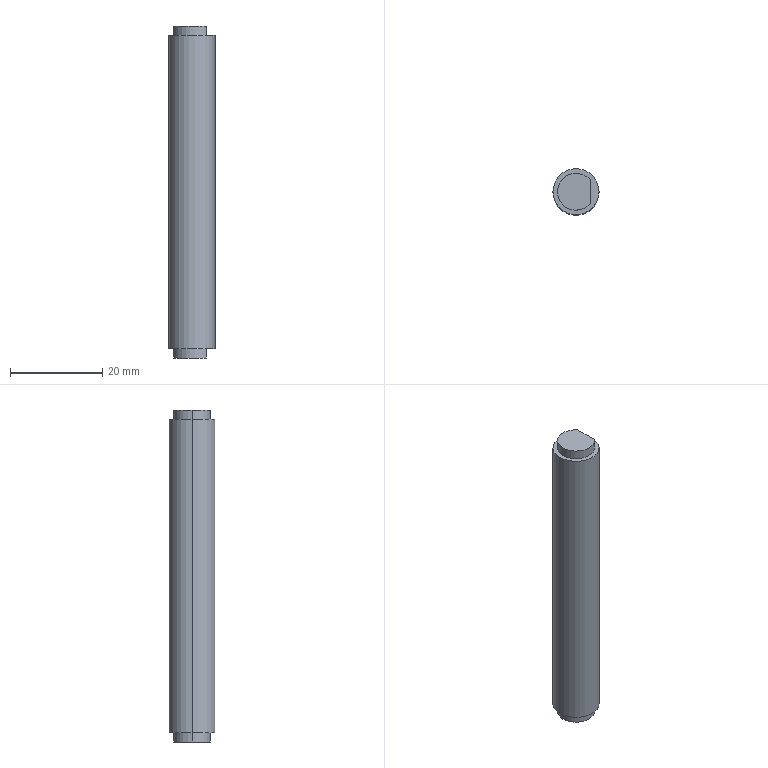Part | STEP file | 1 solid | 12 faces | box 10 x 10 x 72 mm | volume 5529 mm3 | cylinder 6 | plane 6 | commonest cylinder face diameters 8 x4 10 x2
STEP:
#1=CARTESIAN_POINT('',(0.,0.,0.));
#2=DIRECTION('',(0.,0.,1.));
#3=DIRECTION('',(1.,0.,0.));
#4=AXIS2_PLACEMENT_3D('',#1,#2,#3);
#5=CARTESIAN_POINT('',(34.355,10.689,0.));
#6=VERTEX_POINT('',#5);
#7=CARTESIAN_POINT('',(24.355,10.689,0.));
#8=VERTEX_POINT('',#7);
#9=CARTESIAN_POINT('',(29.355,10.689,0.));
#10=DIRECTION('',(0.,0.,1.));
#11=DIRECTION('',(1.,0.,0.));
#12=AXIS2_PLACEMENT_3D('',#9,#10,#11);
#13=CIRCLE('',#12,5.);
#14=CARTESIAN_POINT('',(29.355,10.689,34.));
#15=DIRECTION('',(0.,0.,1.));
#16=DIRECTION('',(1.,0.,0.));
#17=AXIS2_PLACEMENT_3D('',#14,#15,#16);
#18=CYLINDRICAL_SURFACE('',#17,5.);
#19=CARTESIAN_POINT('',(0.,-34.));
#20=DIRECTION('',(1.,0.));
#21=VECTOR('',#20,1.);
#22=LINE('',#19,#21);
#23=(GEOMETRIC_REPRESENTATION_CONTEXT(2)PARAMETRIC_REPRESENTATION_CONTEXT()REPRESENTATION_CONTEXT('',''));
#24=DEFINITIONAL_REPRESENTATION('',(#22),#23);
#25=PCURVE('',#18,#24);
#26=CARTESIAN_POINT('',(29.355,10.689,0.));
#27=DIRECTION('',(0.,0.,1.));
#28=DIRECTION('',(1.,0.,0.));
#29=AXIS2_PLACEMENT_3D('',#26,#27,#28);
#30=PLANE('',#29);
#31=CARTESIAN_POINT('',(0.,0.));
#32=DIRECTION('',(1.,0.));
#33=AXIS2_PLACEMENT_2D('',#31,#32);
#34=CIRCLE('',#33,5.);
#35=(GEOMETRIC_REPRESENTATION_CONTEXT(2)PARAMETRIC_REPRESENTATION_CONTEXT()REPRESENTATION_CONTEXT('',''));
#36=DEFINITIONAL_REPRESENTATION('',(#34),#35);
#37=PCURVE('',#30,#36);
#38=SURFACE_CURVE('',#13,(#25,#37),.PCURVE_S1.);
#39=EDGE_CURVE('',#6,#8,#38,.T.);
#40=ORIENTED_EDGE('',*,*,#39,.T.);
#41=CARTESIAN_POINT('',(24.355,10.689,68.));
#42=VERTEX_POINT('',#41);
#43=CARTESIAN_POINT('',(24.355,10.689,34.));
#44=DIRECTION('',(0.,0.,1.));
#45=VECTOR('',#44,1.);
#46=LINE('',#43,#45);
#47=CARTESIAN_POINT('',(3.142,0.));
#48=DIRECTION('',(0.,1.));
#49=VECTOR('',#48,1.);
#50=LINE('',#47,#49);
#51=(GEOMETRIC_REPRESENTATION_CONTEXT(2)PARAMETRIC_REPRESENTATION_CONTEXT()REPRESENTATION_CONTEXT('',''));
#52=DEFINITIONAL_REPRESENTATION('',(#50),#51);
#53=PCURVE('',#18,#52);
#54=CARTESIAN_POINT('',(29.355,10.689,34.));
#55=DIRECTION('',(0.,0.,1.));
#56=DIRECTION('',(1.,0.,0.));
#57=AXIS2_PLACEMENT_3D('',#54,#55,#56);
#58=CYLINDRICAL_SURFACE('',#57,5.);
#59=CARTESIAN_POINT('',(3.142,0.));
#60=DIRECTION('',(0.,1.));
#61=VECTOR('',#60,1.);
#62=LINE('',#59,#61);
#63=(GEOMETRIC_REPRESENTATION_CONTEXT(2)PARAMETRIC_REPRESENTATION_CONTEXT()REPRESENTATION_CONTEXT('',''));
#64=DEFINITIONAL_REPRESENTATION('',(#62),#63);
#65=PCURVE('',#58,#64);
#66=SURFACE_CURVE('',#46,(#53,#65),.PCURVE_S1.);
#67=EDGE_CURVE('',#8,#42,#66,.T.);
#68=ORIENTED_EDGE('',*,*,#67,.T.);
#69=CARTESIAN_POINT('',(34.355,10.689,68.));
#70=VERTEX_POINT('',#69);
#71=CARTESIAN_POINT('',(29.355,10.689,68.));
#72=DIRECTION('',(0.,0.,-1.));
#73=DIRECTION('',(1.,0.,0.));
#74=AXIS2_PLACEMENT_3D('',#71,#72,#73);
#75=CIRCLE('',#74,5.);
#76=CARTESIAN_POINT('',(6.283,34.));
#77=DIRECTION('',(-1.,0.));
#78=VECTOR('',#77,1.);
#79=LINE('',#76,#78);
#80=(GEOMETRIC_REPRESENTATION_CONTEXT(2)PARAMETRIC_REPRESENTATION_CONTEXT()REPRESENTATION_CONTEXT('',''));
#81=DEFINITIONAL_REPRESENTATION('',(#79),#80);
#82=PCURVE('',#18,#81);
#83=CARTESIAN_POINT('',(29.355,10.689,68.));
#84=DIRECTION('',(0.,0.,1.));
#85=DIRECTION('',(1.,0.,0.));
#86=AXIS2_PLACEMENT_3D('',#83,#84,#85);
#87=PLANE('',#86);
#88=CARTESIAN_POINT('',(5.,0.));
#89=CARTESIAN_POINT('',(5.,-8.66));
#90=CARTESIAN_POINT('',(-2.5,-4.33));
#91=CARTESIAN_POINT('',(-10.,0.));
#92=CARTESIAN_POINT('',(-2.5,4.33));
#93=CARTESIAN_POINT('',(5.,8.66));
#94=CARTESIAN_POINT('',(5.,0.));
#95=(BOUNDED_CURVE()B_SPLINE_CURVE(2,(#88,#89,#90,#91,#92,#93,#94),.UNSPECIFIED.,.T.,.F.)B_SPLINE_CURVE_WITH_KNOTS((1,2,2,2,2,1),(-2.094,0.,2.094,4.189,6.283,8.378),.UNSPECIFIED.)CURVE()GEOMETRIC_REPRESENTATION_ITEM()RATIONAL_B_SPLINE_CURVE((1.,0.5,1.,0.5,1.,0.5,1.))REPRESENTATION_ITEM(''));
#96=(GEOMETRIC_REPRESENTATION_CONTEXT(2)PARAMETRIC_REPRESENTATION_CONTEXT()REPRESENTATION_CONTEXT('',''));
#97=DEFINITIONAL_REPRESENTATION('',(#95),#96);
#98=PCURVE('',#87,#97);
#99=SURFACE_CURVE('',#75,(#82,#98),.PCURVE_S1.);
#100=EDGE_CURVE('',#42,#70,#99,.T.);
#101=ORIENTED_EDGE('',*,*,#100,.T.);
#102=CARTESIAN_POINT('',(34.355,10.689,34.));
#103=DIRECTION('',(0.,0.,1.));
#104=VECTOR('',#103,1.);
#105=LINE('',#102,#104);
#106=CARTESIAN_POINT('',(0.,0.));
#107=DIRECTION('',(0.,1.));
#108=VECTOR('',#107,1.);
#109=LINE('',#106,#108);
#110=(GEOMETRIC_REPRESENTATION_CONTEXT(2)PARAMETRIC_REPRESENTATION_CONTEXT()REPRESENTATION_CONTEXT('',''));
#111=DEFINITIONAL_REPRESENTATION('',(#109),#110);
#112=PCURVE('',#18,#111);
#113=CARTESIAN_POINT('',(6.283,0.));
#114=DIRECTION('',(0.,1.));
#115=VECTOR('',#114,1.);
#116=LINE('',#113,#115);
#117=(GEOMETRIC_REPRESENTATION_CONTEXT(2)PARAMETRIC_REPRESENTATION_CONTEXT()REPRESENTATION_CONTEXT('',''));
#118=DEFINITIONAL_REPRESENTATION('',(#116),#117);
#119=PCURVE('',#58,#118);
#120=SURFACE_CURVE('',#105,(#112,#119),.PCURVE_S1.);
#121=EDGE_CURVE('',#6,#70,#120,.T.);
#122=ORIENTED_EDGE('',*,*,#121,.F.);
#123=EDGE_LOOP('',(#40,#68,#101,#122));
#124=FACE_BOUND('',#123,.T.);
#125=ADVANCED_FACE('',(#124),#18,.T.);
#126=CARTESIAN_POINT('',(32.435,8.137,70.));
#127=VERTEX_POINT('',#126);
#128=CARTESIAN_POINT('',(25.355,10.689,70.));
#129=VERTEX_POINT('',#128);
#130=CARTESIAN_POINT('',(29.355,10.689,70.));
#131=DIRECTION('',(0.,0.,-1.));
#132=DIRECTION('',(-1.,0.,0.));
#133=AXIS2_PLACEMENT_3D('',#130,#131,#132);
#134=CIRCLE('',#133,4.);
#135=CARTESIAN_POINT('',(29.355,10.689,68.));
#136=DIRECTION('',(0.,0.,-1.));
#137=DIRECTION('',(-1.,0.,0.));
#138=AXIS2_PLACEMENT_3D('',#135,#136,#137);
#139=CYLINDRICAL_SURFACE('',#138,4.);
#140=CARTESIAN_POINT('',(0.,-2.));
#141=DIRECTION('',(1.,0.));
#142=VECTOR('',#141,1.);
#143=LINE('',#140,#142);
#144=(GEOMETRIC_REPRESENTATION_CONTEXT(2)PARAMETRIC_REPRESENTATION_CONTEXT()REPRESENTATION_CONTEXT('',''));
#145=DEFINITIONAL_REPRESENTATION('',(#143),#144);
#146=PCURVE('',#139,#145);
#147=CARTESIAN_POINT('',(29.375,10.689,70.));
#148=DIRECTION('',(0.,0.,1.));
#149=DIRECTION('',(1.,0.,0.));
#150=AXIS2_PLACEMENT_3D('',#147,#148,#149);
#151=PLANE('',#150);
#152=CARTESIAN_POINT('',(-4.021,0.));
#153=CARTESIAN_POINT('',(-4.021,6.928));
#154=CARTESIAN_POINT('',(1.979,3.464));
#155=CARTESIAN_POINT('',(7.979,0.));
#156=CARTESIAN_POINT('',(1.979,-3.464));
#157=CARTESIAN_POINT('',(-4.021,-6.928));
#158=CARTESIAN_POINT('',(-4.021,0.));
#159=(BOUNDED_CURVE()B_SPLINE_CURVE(2,(#152,#153,#154,#155,#156,#157,#158),.UNSPECIFIED.,.T.,.F.)B_SPLINE_CURVE_WITH_KNOTS((1,2,2,2,2,1),(-2.094,0.,2.094,4.189,6.283,8.378),.UNSPECIFIED.)CURVE()GEOMETRIC_REPRESENTATION_ITEM()RATIONAL_B_SPLINE_CURVE((1.,0.5,1.,0.5,1.,0.5,1.))REPRESENTATION_ITEM(''));
#160=(GEOMETRIC_REPRESENTATION_CONTEXT(2)PARAMETRIC_REPRESENTATION_CONTEXT()REPRESENTATION_CONTEXT('',''));
#161=DEFINITIONAL_REPRESENTATION('',(#159),#160);
#162=PCURVE('',#151,#161);
#163=SURFACE_CURVE('',#134,(#146,#162),.PCURVE_S1.);
#164=EDGE_CURVE('',#127,#129,#163,.T.);
#165=ORIENTED_EDGE('',*,*,#164,.T.);
#166=CARTESIAN_POINT('',(25.355,10.689,68.));
#167=VERTEX_POINT('',#166);
#168=CARTESIAN_POINT('',(25.355,10.689,68.));
#169=DIRECTION('',(0.,0.,-1.));
#170=VECTOR('',#169,1.);
#171=LINE('',#168,#170);
#172=CARTESIAN_POINT('',(6.283,0.));
#173=DIRECTION('',(0.,1.));
#174=VECTOR('',#173,1.);
#175=LINE('',#172,#174);
#176=(GEOMETRIC_REPRESENTATION_CONTEXT(2)PARAMETRIC_REPRESENTATION_CONTEXT()REPRESENTATION_CONTEXT('',''));
#177=DEFINITIONAL_REPRESENTATION('',(#175),#176);
#178=PCURVE('',#139,#177);
#179=CARTESIAN_POINT('',(29.355,10.689,68.));
#180=DIRECTION('',(0.,0.,-1.));
#181=DIRECTION('',(-1.,0.,0.));
#182=AXIS2_PLACEMENT_3D('',#179,#180,#181);
#183=CYLINDRICAL_SURFACE('',#182,4.);
#184=CARTESIAN_POINT('',(0.,0.));
#185=DIRECTION('',(0.,1.));
#186=VECTOR('',#185,1.);
#187=LINE('',#184,#186);
#188=(GEOMETRIC_REPRESENTATION_CONTEXT(2)PARAMETRIC_REPRESENTATION_CONTEXT()REPRESENTATION_CONTEXT('',''));
#189=DEFINITIONAL_REPRESENTATION('',(#187),#188);
#190=PCURVE('',#183,#189);
#191=SURFACE_CURVE('',#171,(#178,#190),.PCURVE_S1.);
#192=EDGE_CURVE('',#129,#167,#191,.T.);
#193=ORIENTED_EDGE('',*,*,#192,.T.);
#194=CARTESIAN_POINT('',(32.435,8.137,68.));
#195=VERTEX_POINT('',#194);
#196=CARTESIAN_POINT('',(29.355,10.689,68.));
#197=DIRECTION('',(0.,0.,-1.));
#198=DIRECTION('',(-1.,0.,0.));
#199=AXIS2_PLACEMENT_3D('',#196,#197,#198);
#200=CIRCLE('',#199,4.);
#201=CARTESIAN_POINT('',(0.,0.));
#202=DIRECTION('',(1.,0.));
#203=VECTOR('',#202,1.);
#204=LINE('',#201,#203);
#205=(GEOMETRIC_REPRESENTATION_CONTEXT(2)PARAMETRIC_REPRESENTATION_CONTEXT()REPRESENTATION_CONTEXT('',''));
#206=DEFINITIONAL_REPRESENTATION('',(#204),#205);
#207=PCURVE('',#139,#206);
#208=CARTESIAN_POINT('',(-4.,0.));
#209=CARTESIAN_POINT('',(-4.,6.928));
#210=CARTESIAN_POINT('',(2.,3.464));
#211=CARTESIAN_POINT('',(8.,0.));
#212=CARTESIAN_POINT('',(2.,-3.464));
#213=CARTESIAN_POINT('',(-4.,-6.928));
#214=CARTESIAN_POINT('',(-4.,0.));
#215=(BOUNDED_CURVE()B_SPLINE_CURVE(2,(#208,#209,#210,#211,#212,#213,#214),.UNSPECIFIED.,.T.,.F.)B_SPLINE_CURVE_WITH_KNOTS((1,2,2,2,2,1),(-2.094,0.,2.094,4.189,6.283,8.378),.UNSPECIFIED.)CURVE()GEOMETRIC_REPRESENTATION_ITEM()RATIONAL_B_SPLINE_CURVE((1.,0.5,1.,0.5,1.,0.5,1.))REPRESENTATION_ITEM(''));
#216=(GEOMETRIC_REPRESENTATION_CONTEXT(2)PARAMETRIC_REPRESENTATION_CONTEXT()REPRESENTATION_CONTEXT('',''));
#217=DEFINITIONAL_REPRESENTATION('',(#215),#216);
#218=PCURVE('',#87,#217);
#219=SURFACE_CURVE('',#200,(#207,#218),.PCURVE_S1.);
#220=EDGE_CURVE('',#195,#167,#219,.T.);
#221=ORIENTED_EDGE('',*,*,#220,.F.);
#222=CARTESIAN_POINT('',(32.435,8.137,68.));
#223=DIRECTION('',(0.,0.,1.));
#224=VECTOR('',#223,1.);
#225=LINE('',#222,#224);
#226=CARTESIAN_POINT('',(3.833,0.));
#227=DIRECTION('',(0.,-1.));
#228=VECTOR('',#227,1.);
#229=LINE('',#226,#228);
#230=(GEOMETRIC_REPRESENTATION_CONTEXT(2)PARAMETRIC_REPRESENTATION_CONTEXT()REPRESENTATION_CONTEXT('',''));
#231=DEFINITIONAL_REPRESENTATION('',(#229),#230);
#232=PCURVE('',#139,#231);
#233=CARTESIAN_POINT('',(32.435,13.24,68.));
#234=DIRECTION('',(-1.,0.,0.));
#235=DIRECTION('',(0.,-1.,0.));
#236=AXIS2_PLACEMENT_3D('',#233,#234,#235);
#237=PLANE('',#236);
#238=CARTESIAN_POINT('',(5.103,0.));
#239=DIRECTION('',(0.,1.));
#240=VECTOR('',#239,1.);
#241=LINE('',#238,#240);
#242=(GEOMETRIC_REPRESENTATION_CONTEXT(2)PARAMETRIC_REPRESENTATION_CONTEXT()REPRESENTATION_CONTEXT('',''));
#243=DEFINITIONAL_REPRESENTATION('',(#241),#242);
#244=PCURVE('',#237,#243);
#245=SURFACE_CURVE('',#225,(#232,#244),.PCURVE_S1.);
#246=EDGE_CURVE('',#195,#127,#245,.T.);
#247=ORIENTED_EDGE('',*,*,#246,.T.);
#248=EDGE_LOOP('',(#165,#193,#221,#247));
#249=FACE_BOUND('',#248,.T.);
#250=ADVANCED_FACE('',(#249),#139,.T.);
#251=CARTESIAN_POINT('',(32.435,8.137,0.));
#252=VERTEX_POINT('',#251);
#253=CARTESIAN_POINT('',(25.355,10.689,0.));
#254=VERTEX_POINT('',#253);
#255=CARTESIAN_POINT('',(29.355,10.689,0.));
#256=DIRECTION('',(0.,0.,-1.));
#257=DIRECTION('',(-1.,0.,0.));
#258=AXIS2_PLACEMENT_3D('',#255,#256,#257);
#259=CIRCLE('',#258,4.);
#260=CARTESIAN_POINT('',(29.355,10.689,0.));
#261=DIRECTION('',(0.,0.,-1.));
#262=DIRECTION('',(-1.,0.,0.));
#263=AXIS2_PLACEMENT_3D('',#260,#261,#262);
#264=CYLINDRICAL_SURFACE('',#263,4.);
#265=CARTESIAN_POINT('',(0.,0.));
#266=DIRECTION('',(1.,0.));
#267=VECTOR('',#266,1.);
#268=LINE('',#265,#267);
#269=(GEOMETRIC_REPRESENTATION_CONTEXT(2)PARAMETRIC_REPRESENTATION_CONTEXT()REPRESENTATION_CONTEXT('',''));
#270=DEFINITIONAL_REPRESENTATION('',(#268),#269);
#271=PCURVE('',#264,#270);
#272=CARTESIAN_POINT('',(-4.,0.));
#273=CARTESIAN_POINT('',(-4.,6.928));
#274=CARTESIAN_POINT('',(2.,3.464));
#275=CARTESIAN_POINT('',(8.,0.));
#276=CARTESIAN_POINT('',(2.,-3.464));
#277=CARTESIAN_POINT('',(-4.,-6.928));
#278=CARTESIAN_POINT('',(-4.,0.));
#279=(BOUNDED_CURVE()B_SPLINE_CURVE(2,(#272,#273,#274,#275,#276,#277,#278),.UNSPECIFIED.,.T.,.F.)B_SPLINE_CURVE_WITH_KNOTS((1,2,2,2,2,1),(-2.094,0.,2.094,4.189,6.283,8.378),.UNSPECIFIED.)CURVE()GEOMETRIC_REPRESENTATION_ITEM()RATIONAL_B_SPLINE_CURVE((1.,0.5,1.,0.5,1.,0.5,1.))REPRESENTATION_ITEM(''));
#280=(GEOMETRIC_REPRESENTATION_CONTEXT(2)PARAMETRIC_REPRESENTATION_CONTEXT()REPRESENTATION_CONTEXT('',''));
#281=DEFINITIONAL_REPRESENTATION('',(#279),#280);
#282=PCURVE('',#30,#281);
#283=SURFACE_CURVE('',#259,(#271,#282),.PCURVE_S1.);
#284=EDGE_CURVE('',#252,#254,#283,.T.);
#285=ORIENTED_EDGE('',*,*,#284,.T.);
#286=CARTESIAN_POINT('',(25.355,10.689,-2.));
#287=VERTEX_POINT('',#286);
#288=CARTESIAN_POINT('',(25.355,10.689,0.));
#289=DIRECTION('',(0.,0.,-1.));
#290=VECTOR('',#289,1.);
#291=LINE('',#288,#290);
#292=CARTESIAN_POINT('',(6.283,0.));
#293=DIRECTION('',(0.,1.));
#294=VECTOR('',#293,1.);
#295=LINE('',#292,#294);
#296=(GEOMETRIC_REPRESENTATION_CONTEXT(2)PARAMETRIC_REPRESENTATION_CONTEXT()REPRESENTATION_CONTEXT('',''));
#297=DEFINITIONAL_REPRESENTATION('',(#295),#296);
#298=PCURVE('',#264,#297);
#299=CARTESIAN_POINT('',(29.355,10.689,0.));
#300=DIRECTION('',(0.,0.,-1.));
#301=DIRECTION('',(-1.,0.,0.));
#302=AXIS2_PLACEMENT_3D('',#299,#300,#301);
#303=CYLINDRICAL_SURFACE('',#302,4.);
#304=CARTESIAN_POINT('',(0.,0.));
#305=DIRECTION('',(0.,1.));
#306=VECTOR('',#305,1.);
#307=LINE('',#304,#306);
#308=(GEOMETRIC_REPRESENTATION_CONTEXT(2)PARAMETRIC_REPRESENTATION_CONTEXT()REPRESENTATION_CONTEXT('',''));
#309=DEFINITIONAL_REPRESENTATION('',(#307),#308);
#310=PCURVE('',#303,#309);
#311=SURFACE_CURVE('',#291,(#298,#310),.PCURVE_S1.);
#312=EDGE_CURVE('',#254,#287,#311,.T.);
#313=ORIENTED_EDGE('',*,*,#312,.T.);
#314=CARTESIAN_POINT('',(32.435,8.137,-2.));
#315=VERTEX_POINT('',#314);
#316=CARTESIAN_POINT('',(29.355,10.689,-2.));
#317=DIRECTION('',(0.,0.,1.));
#318=DIRECTION('',(-1.,0.,0.));
#319=AXIS2_PLACEMENT_3D('',#316,#317,#318);
#320=CIRCLE('',#319,4.);
#321=CARTESIAN_POINT('',(6.283,2.));
#322=DIRECTION('',(-1.,0.));
#323=VECTOR('',#322,1.);
#324=LINE('',#321,#323);
#325=(GEOMETRIC_REPRESENTATION_CONTEXT(2)PARAMETRIC_REPRESENTATION_CONTEXT()REPRESENTATION_CONTEXT('',''));
#326=DEFINITIONAL_REPRESENTATION('',(#324),#325);
#327=PCURVE('',#264,#326);
#328=CARTESIAN_POINT('',(29.375,10.689,-2.));
#329=DIRECTION('',(0.,0.,1.));
#330=DIRECTION('',(1.,0.,0.));
#331=AXIS2_PLACEMENT_3D('',#328,#329,#330);
#332=PLANE('',#331);
#333=CARTESIAN_POINT('',(-0.02072,0.));
#334=DIRECTION('',(-1.,0.));
#335=AXIS2_PLACEMENT_2D('',#333,#334);
#336=CIRCLE('',#335,4.);
#337=(GEOMETRIC_REPRESENTATION_CONTEXT(2)PARAMETRIC_REPRESENTATION_CONTEXT()REPRESENTATION_CONTEXT('',''));
#338=DEFINITIONAL_REPRESENTATION('',(#336),#337);
#339=PCURVE('',#332,#338);
#340=SURFACE_CURVE('',#320,(#327,#339),.PCURVE_S1.);
#341=EDGE_CURVE('',#287,#315,#340,.T.);
#342=ORIENTED_EDGE('',*,*,#341,.T.);
#343=CARTESIAN_POINT('',(32.435,8.137,0.));
#344=DIRECTION('',(0.,0.,-1.));
#345=VECTOR('',#344,1.);
#346=LINE('',#343,#345);
#347=CARTESIAN_POINT('',(3.833,0.));
#348=DIRECTION('',(0.,1.));
#349=VECTOR('',#348,1.);
#350=LINE('',#347,#349);
#351=(GEOMETRIC_REPRESENTATION_CONTEXT(2)PARAMETRIC_REPRESENTATION_CONTEXT()REPRESENTATION_CONTEXT('',''));
#352=DEFINITIONAL_REPRESENTATION('',(#350),#351);
#353=PCURVE('',#264,#352);
#354=CARTESIAN_POINT('',(32.435,13.24,0.));
#355=DIRECTION('',(1.,0.,0.));
#356=DIRECTION('',(0.,1.,0.));
#357=AXIS2_PLACEMENT_3D('',#354,#355,#356);
#358=PLANE('',#357);
#359=CARTESIAN_POINT('',(-5.103,0.));
#360=DIRECTION('',(0.,-1.));
#361=VECTOR('',#360,1.);
#362=LINE('',#359,#361);
#363=(GEOMETRIC_REPRESENTATION_CONTEXT(2)PARAMETRIC_REPRESENTATION_CONTEXT()REPRESENTATION_CONTEXT('',''));
#364=DEFINITIONAL_REPRESENTATION('',(#362),#363);
#365=PCURVE('',#358,#364);
#366=SURFACE_CURVE('',#346,(#353,#365),.PCURVE_S1.);
#367=EDGE_CURVE('',#252,#315,#366,.T.);
#368=ORIENTED_EDGE('',*,*,#367,.F.);
#369=EDGE_LOOP('',(#285,#313,#342,#368));
#370=FACE_BOUND('',#369,.T.);
#371=ADVANCED_FACE('',(#370),#264,.T.);
#372=ORIENTED_EDGE('',*,*,#67,.F.);
#373=CARTESIAN_POINT('',(29.355,10.689,0.));
#374=DIRECTION('',(0.,0.,1.));
#375=DIRECTION('',(1.,0.,0.));
#376=AXIS2_PLACEMENT_3D('',#373,#374,#375);
#377=CIRCLE('',#376,5.);
#378=CARTESIAN_POINT('',(0.,-34.));
#379=DIRECTION('',(1.,0.));
#380=VECTOR('',#379,1.);
#381=LINE('',#378,#380);
#382=(GEOMETRIC_REPRESENTATION_CONTEXT(2)PARAMETRIC_REPRESENTATION_CONTEXT()REPRESENTATION_CONTEXT('',''));
#383=DEFINITIONAL_REPRESENTATION('',(#381),#382);
#384=PCURVE('',#58,#383);
#385=CARTESIAN_POINT('',(0.,0.));
#386=DIRECTION('',(1.,0.));
#387=AXIS2_PLACEMENT_2D('',#385,#386);
#388=CIRCLE('',#387,5.);
#389=(GEOMETRIC_REPRESENTATION_CONTEXT(2)PARAMETRIC_REPRESENTATION_CONTEXT()REPRESENTATION_CONTEXT('',''));
#390=DEFINITIONAL_REPRESENTATION('',(#388),#389);
#391=PCURVE('',#30,#390);
#392=SURFACE_CURVE('',#377,(#384,#391),.PCURVE_S1.);
#393=EDGE_CURVE('',#8,#6,#392,.T.);
#394=ORIENTED_EDGE('',*,*,#393,.T.);
#395=ORIENTED_EDGE('',*,*,#121,.T.);
#396=CARTESIAN_POINT('',(29.355,10.689,68.));
#397=DIRECTION('',(0.,0.,-1.));
#398=DIRECTION('',(1.,0.,0.));
#399=AXIS2_PLACEMENT_3D('',#396,#397,#398);
#400=CIRCLE('',#399,5.);
#401=CARTESIAN_POINT('',(6.283,34.));
#402=DIRECTION('',(-1.,0.));
#403=VECTOR('',#402,1.);
#404=LINE('',#401,#403);
#405=(GEOMETRIC_REPRESENTATION_CONTEXT(2)PARAMETRIC_REPRESENTATION_CONTEXT()REPRESENTATION_CONTEXT('',''));
#406=DEFINITIONAL_REPRESENTATION('',(#404),#405);
#407=PCURVE('',#58,#406);
#408=CARTESIAN_POINT('',(5.,0.));
#409=CARTESIAN_POINT('',(5.,-8.66));
#410=CARTESIAN_POINT('',(-2.5,-4.33));
#411=CARTESIAN_POINT('',(-10.,0.));
#412=CARTESIAN_POINT('',(-2.5,4.33));
#413=CARTESIAN_POINT('',(5.,8.66));
#414=CARTESIAN_POINT('',(5.,0.));
#415=(BOUNDED_CURVE()B_SPLINE_CURVE(2,(#408,#409,#410,#411,#412,#413,#414),.UNSPECIFIED.,.T.,.F.)B_SPLINE_CURVE_WITH_KNOTS((1,2,2,2,2,1),(-2.094,0.,2.094,4.189,6.283,8.378),.UNSPECIFIED.)CURVE()GEOMETRIC_REPRESENTATION_ITEM()RATIONAL_B_SPLINE_CURVE((1.,0.5,1.,0.5,1.,0.5,1.))REPRESENTATION_ITEM(''));
#416=(GEOMETRIC_REPRESENTATION_CONTEXT(2)PARAMETRIC_REPRESENTATION_CONTEXT()REPRESENTATION_CONTEXT('',''));
#417=DEFINITIONAL_REPRESENTATION('',(#415),#416);
#418=PCURVE('',#87,#417);
#419=SURFACE_CURVE('',#400,(#407,#418),.PCURVE_S1.);
#420=EDGE_CURVE('',#70,#42,#419,.T.);
#421=ORIENTED_EDGE('',*,*,#420,.T.);
#422=EDGE_LOOP('',(#372,#394,#395,#421));
#423=FACE_BOUND('',#422,.T.);
#424=ADVANCED_FACE('',(#423),#58,.T.);
#425=ORIENTED_EDGE('',*,*,#420,.F.);
#426=ORIENTED_EDGE('',*,*,#100,.F.);
#427=EDGE_LOOP('',(#425,#426));
#428=FACE_BOUND('',#427,.T.);
#429=CARTESIAN_POINT('',(32.435,13.24,68.));
#430=VERTEX_POINT('',#429);
#431=CARTESIAN_POINT('',(32.435,10.689,68.));
#432=DIRECTION('',(0.,-1.,0.));
#433=VECTOR('',#432,1.);
#434=LINE('',#431,#433);
#435=CARTESIAN_POINT('',(3.08,0.));
#436=DIRECTION('',(0.,-1.));
#437=VECTOR('',#436,1.);
#438=LINE('',#435,#437);
#439=(GEOMETRIC_REPRESENTATION_CONTEXT(2)PARAMETRIC_REPRESENTATION_CONTEXT()REPRESENTATION_CONTEXT('',''));
#440=DEFINITIONAL_REPRESENTATION('',(#438),#439);
#441=PCURVE('',#87,#440);
#442=CARTESIAN_POINT('',(2.552,0.));
#443=DIRECTION('',(1.,0.));
#444=VECTOR('',#443,1.);
#445=LINE('',#442,#444);
#446=(GEOMETRIC_REPRESENTATION_CONTEXT(2)PARAMETRIC_REPRESENTATION_CONTEXT()REPRESENTATION_CONTEXT('',''));
#447=DEFINITIONAL_REPRESENTATION('',(#445),#446);
#448=PCURVE('',#237,#447);
#449=SURFACE_CURVE('',#434,(#441,#448),.PCURVE_S1.);
#450=EDGE_CURVE('',#430,#195,#449,.T.);
#451=ORIENTED_EDGE('',*,*,#450,.T.);
#452=ORIENTED_EDGE('',*,*,#220,.T.);
#453=CARTESIAN_POINT('',(29.355,10.689,68.));
#454=DIRECTION('',(0.,0.,-1.));
#455=DIRECTION('',(-1.,0.,0.));
#456=AXIS2_PLACEMENT_3D('',#453,#454,#455);
#457=CIRCLE('',#456,4.);
#458=CARTESIAN_POINT('',(-4.,0.));
#459=CARTESIAN_POINT('',(-4.,6.928));
#460=CARTESIAN_POINT('',(2.,3.464));
#461=CARTESIAN_POINT('',(8.,0.));
#462=CARTESIAN_POINT('',(2.,-3.464));
#463=CARTESIAN_POINT('',(-4.,-6.928));
#464=CARTESIAN_POINT('',(-4.,0.));
#465=(BOUNDED_CURVE()B_SPLINE_CURVE(2,(#458,#459,#460,#461,#462,#463,#464),.UNSPECIFIED.,.T.,.F.)B_SPLINE_CURVE_WITH_KNOTS((1,2,2,2,2,1),(-2.094,0.,2.094,4.189,6.283,8.378),.UNSPECIFIED.)CURVE()GEOMETRIC_REPRESENTATION_ITEM()RATIONAL_B_SPLINE_CURVE((1.,0.5,1.,0.5,1.,0.5,1.))REPRESENTATION_ITEM(''));
#466=(GEOMETRIC_REPRESENTATION_CONTEXT(2)PARAMETRIC_REPRESENTATION_CONTEXT()REPRESENTATION_CONTEXT('',''));
#467=DEFINITIONAL_REPRESENTATION('',(#465),#466);
#468=PCURVE('',#87,#467);
#469=CARTESIAN_POINT('',(0.,0.));
#470=DIRECTION('',(1.,0.));
#471=VECTOR('',#470,1.);
#472=LINE('',#469,#471);
#473=(GEOMETRIC_REPRESENTATION_CONTEXT(2)PARAMETRIC_REPRESENTATION_CONTEXT()REPRESENTATION_CONTEXT('',''));
#474=DEFINITIONAL_REPRESENTATION('',(#472),#473);
#475=PCURVE('',#183,#474);
#476=SURFACE_CURVE('',#457,(#468,#475),.PCURVE_S1.);
#477=EDGE_CURVE('',#167,#430,#476,.T.);
#478=ORIENTED_EDGE('',*,*,#477,.T.);
#479=EDGE_LOOP('',(#451,#452,#478));
#480=FACE_BOUND('',#479,.T.);
#481=ADVANCED_FACE('',(#428,#480),#87,.T.);
#482=ORIENTED_EDGE('',*,*,#39,.F.);
#483=ORIENTED_EDGE('',*,*,#393,.F.);
#484=EDGE_LOOP('',(#482,#483));
#485=FACE_BOUND('',#484,.T.);
#486=ORIENTED_EDGE('',*,*,#284,.F.);
#487=CARTESIAN_POINT('',(32.435,13.24,0.));
#488=VERTEX_POINT('',#487);
#489=CARTESIAN_POINT('',(32.435,10.689,0.));
#490=DIRECTION('',(0.,-1.,0.));
#491=VECTOR('',#490,1.);
#492=LINE('',#489,#491);
#493=CARTESIAN_POINT('',(3.08,0.));
#494=DIRECTION('',(0.,-1.));
#495=VECTOR('',#494,1.);
#496=LINE('',#493,#495);
#497=(GEOMETRIC_REPRESENTATION_CONTEXT(2)PARAMETRIC_REPRESENTATION_CONTEXT()REPRESENTATION_CONTEXT('',''));
#498=DEFINITIONAL_REPRESENTATION('',(#496),#497);
#499=PCURVE('',#30,#498);
#500=CARTESIAN_POINT('',(-2.552,0.));
#501=DIRECTION('',(-1.,0.));
#502=VECTOR('',#501,1.);
#503=LINE('',#500,#502);
#504=(GEOMETRIC_REPRESENTATION_CONTEXT(2)PARAMETRIC_REPRESENTATION_CONTEXT()REPRESENTATION_CONTEXT('',''));
#505=DEFINITIONAL_REPRESENTATION('',(#503),#504);
#506=PCURVE('',#358,#505);
#507=SURFACE_CURVE('',#492,(#499,#506),.PCURVE_S1.);
#508=EDGE_CURVE('',#488,#252,#507,.T.);
#509=ORIENTED_EDGE('',*,*,#508,.F.);
#510=CARTESIAN_POINT('',(29.355,10.689,0.));
#511=DIRECTION('',(0.,0.,-1.));
#512=DIRECTION('',(-1.,0.,0.));
#513=AXIS2_PLACEMENT_3D('',#510,#511,#512);
#514=CIRCLE('',#513,4.);
#515=CARTESIAN_POINT('',(-4.,0.));
#516=CARTESIAN_POINT('',(-4.,6.928));
#517=CARTESIAN_POINT('',(2.,3.464));
#518=CARTESIAN_POINT('',(8.,0.));
#519=CARTESIAN_POINT('',(2.,-3.464));
#520=CARTESIAN_POINT('',(-4.,-6.928));
#521=CARTESIAN_POINT('',(-4.,0.));
#522=(BOUNDED_CURVE()B_SPLINE_CURVE(2,(#515,#516,#517,#518,#519,#520,#521),.UNSPECIFIED.,.T.,.F.)B_SPLINE_CURVE_WITH_KNOTS((1,2,2,2,2,1),(-2.094,0.,2.094,4.189,6.283,8.378),.UNSPECIFIED.)CURVE()GEOMETRIC_REPRESENTATION_ITEM()RATIONAL_B_SPLINE_CURVE((1.,0.5,1.,0.5,1.,0.5,1.))REPRESENTATION_ITEM(''));
#523=(GEOMETRIC_REPRESENTATION_CONTEXT(2)PARAMETRIC_REPRESENTATION_CONTEXT()REPRESENTATION_CONTEXT('',''));
#524=DEFINITIONAL_REPRESENTATION('',(#522),#523);
#525=PCURVE('',#30,#524);
#526=CARTESIAN_POINT('',(0.,0.));
#527=DIRECTION('',(1.,0.));
#528=VECTOR('',#527,1.);
#529=LINE('',#526,#528);
#530=(GEOMETRIC_REPRESENTATION_CONTEXT(2)PARAMETRIC_REPRESENTATION_CONTEXT()REPRESENTATION_CONTEXT('',''));
#531=DEFINITIONAL_REPRESENTATION('',(#529),#530);
#532=PCURVE('',#303,#531);
#533=SURFACE_CURVE('',#514,(#525,#532),.PCURVE_S1.);
#534=EDGE_CURVE('',#254,#488,#533,.T.);
#535=ORIENTED_EDGE('',*,*,#534,.F.);
#536=EDGE_LOOP('',(#486,#509,#535));
#537=FACE_BOUND('',#536,.T.);
#538=ADVANCED_FACE('',(#485,#537),#30,.F.);
#539=ORIENTED_EDGE('',*,*,#192,.F.);
#540=CARTESIAN_POINT('',(32.435,13.24,70.));
#541=VERTEX_POINT('',#540);
#542=CARTESIAN_POINT('',(29.355,10.689,70.));
#543=DIRECTION('',(0.,0.,-1.));
#544=DIRECTION('',(-1.,0.,0.));
#545=AXIS2_PLACEMENT_3D('',#542,#543,#544);
#546=CIRCLE('',#545,4.);
#547=CARTESIAN_POINT('',(0.,-2.));
#548=DIRECTION('',(1.,0.));
#549=VECTOR('',#548,1.);
#550=LINE('',#547,#549);
#551=(GEOMETRIC_REPRESENTATION_CONTEXT(2)PARAMETRIC_REPRESENTATION_CONTEXT()REPRESENTATION_CONTEXT('',''));
#552=DEFINITIONAL_REPRESENTATION('',(#550),#551);
#553=PCURVE('',#183,#552);
#554=CARTESIAN_POINT('',(-4.021,0.));
#555=CARTESIAN_POINT('',(-4.021,6.928));
#556=CARTESIAN_POINT('',(1.979,3.464));
#557=CARTESIAN_POINT('',(7.979,0.));
#558=CARTESIAN_POINT('',(1.979,-3.464));
#559=CARTESIAN_POINT('',(-4.021,-6.928));
#560=CARTESIAN_POINT('',(-4.021,0.));
#561=(BOUNDED_CURVE()B_SPLINE_CURVE(2,(#554,#555,#556,#557,#558,#559,#560),.UNSPECIFIED.,.T.,.F.)B_SPLINE_CURVE_WITH_KNOTS((1,2,2,2,2,1),(-2.094,0.,2.094,4.189,6.283,8.378),.UNSPECIFIED.)CURVE()GEOMETRIC_REPRESENTATION_ITEM()RATIONAL_B_SPLINE_CURVE((1.,0.5,1.,0.5,1.,0.5,1.))REPRESENTATION_ITEM(''));
#562=(GEOMETRIC_REPRESENTATION_CONTEXT(2)PARAMETRIC_REPRESENTATION_CONTEXT()REPRESENTATION_CONTEXT('',''));
#563=DEFINITIONAL_REPRESENTATION('',(#561),#562);
#564=PCURVE('',#151,#563);
#565=SURFACE_CURVE('',#546,(#553,#564),.PCURVE_S1.);
#566=EDGE_CURVE('',#129,#541,#565,.T.);
#567=ORIENTED_EDGE('',*,*,#566,.T.);
#568=CARTESIAN_POINT('',(32.435,13.24,68.));
#569=DIRECTION('',(0.,0.,-1.));
#570=VECTOR('',#569,1.);
#571=LINE('',#568,#570);
#572=CARTESIAN_POINT('',(2.45,0.));
#573=DIRECTION('',(0.,1.));
#574=VECTOR('',#573,1.);
#575=LINE('',#572,#574);
#576=(GEOMETRIC_REPRESENTATION_CONTEXT(2)PARAMETRIC_REPRESENTATION_CONTEXT()REPRESENTATION_CONTEXT('',''));
#577=DEFINITIONAL_REPRESENTATION('',(#575),#576);
#578=PCURVE('',#183,#577);
#579=CARTESIAN_POINT('',(0.,0.));
#580=DIRECTION('',(0.,-1.));
#581=VECTOR('',#580,1.);
#582=LINE('',#579,#581);
#583=(GEOMETRIC_REPRESENTATION_CONTEXT(2)PARAMETRIC_REPRESENTATION_CONTEXT()REPRESENTATION_CONTEXT('',''));
#584=DEFINITIONAL_REPRESENTATION('',(#582),#583);
#585=PCURVE('',#237,#584);
#586=SURFACE_CURVE('',#571,(#578,#585),.PCURVE_S1.);
#587=EDGE_CURVE('',#541,#430,#586,.T.);
#588=ORIENTED_EDGE('',*,*,#587,.T.);
#589=ORIENTED_EDGE('',*,*,#477,.F.);
#590=EDGE_LOOP('',(#539,#567,#588,#589));
#591=FACE_BOUND('',#590,.T.);
#592=ADVANCED_FACE('',(#591),#183,.T.);
#593=ORIENTED_EDGE('',*,*,#587,.F.);
#594=CARTESIAN_POINT('',(32.435,13.24,70.));
#595=DIRECTION('',(0.,1.,0.));
#596=VECTOR('',#595,1.);
#597=LINE('',#594,#596);
#598=CARTESIAN_POINT('',(0.,2.));
#599=DIRECTION('',(-1.,0.));
#600=VECTOR('',#599,1.);
#601=LINE('',#598,#600);
#602=(GEOMETRIC_REPRESENTATION_CONTEXT(2)PARAMETRIC_REPRESENTATION_CONTEXT()REPRESENTATION_CONTEXT('',''));
#603=DEFINITIONAL_REPRESENTATION('',(#601),#602);
#604=PCURVE('',#237,#603);
#605=CARTESIAN_POINT('',(3.06,2.552));
#606=DIRECTION('',(0.,1.));
#607=VECTOR('',#606,1.);
#608=LINE('',#605,#607);
#609=(GEOMETRIC_REPRESENTATION_CONTEXT(2)PARAMETRIC_REPRESENTATION_CONTEXT()REPRESENTATION_CONTEXT('',''));
#610=DEFINITIONAL_REPRESENTATION('',(#608),#609);
#611=PCURVE('',#151,#610);
#612=SURFACE_CURVE('',#597,(#604,#611),.PCURVE_S1.);
#613=EDGE_CURVE('',#127,#541,#612,.T.);
#614=ORIENTED_EDGE('',*,*,#613,.F.);
#615=ORIENTED_EDGE('',*,*,#246,.F.);
#616=ORIENTED_EDGE('',*,*,#450,.F.);
#617=EDGE_LOOP('',(#593,#614,#615,#616));
#618=FACE_BOUND('',#617,.T.);
#619=ADVANCED_FACE('',(#618),#237,.F.);
#620=CARTESIAN_POINT('',(32.435,13.24,-2.));
#621=VERTEX_POINT('',#620);
#622=CARTESIAN_POINT('',(32.435,13.24,-2.));
#623=DIRECTION('',(0.,1.,0.));
#624=VECTOR('',#623,1.);
#625=LINE('',#622,#624);
#626=CARTESIAN_POINT('',(0.,-2.));
#627=DIRECTION('',(1.,0.));
#628=VECTOR('',#627,1.);
#629=LINE('',#626,#628);
#630=(GEOMETRIC_REPRESENTATION_CONTEXT(2)PARAMETRIC_REPRESENTATION_CONTEXT()REPRESENTATION_CONTEXT('',''));
#631=DEFINITIONAL_REPRESENTATION('',(#629),#630);
#632=PCURVE('',#358,#631);
#633=CARTESIAN_POINT('',(3.06,2.552));
#634=DIRECTION('',(0.,1.));
#635=VECTOR('',#634,1.);
#636=LINE('',#633,#635);
#637=(GEOMETRIC_REPRESENTATION_CONTEXT(2)PARAMETRIC_REPRESENTATION_CONTEXT()REPRESENTATION_CONTEXT('',''));
#638=DEFINITIONAL_REPRESENTATION('',(#636),#637);
#639=PCURVE('',#332,#638);
#640=SURFACE_CURVE('',#625,(#632,#639),.PCURVE_S1.);
#641=EDGE_CURVE('',#315,#621,#640,.T.);
#642=ORIENTED_EDGE('',*,*,#641,.T.);
#643=CARTESIAN_POINT('',(32.435,13.24,0.));
#644=DIRECTION('',(0.,0.,1.));
#645=VECTOR('',#644,1.);
#646=LINE('',#643,#645);
#647=CARTESIAN_POINT('',(0.,0.));
#648=DIRECTION('',(0.,1.));
#649=VECTOR('',#648,1.);
#650=LINE('',#647,#649);
#651=(GEOMETRIC_REPRESENTATION_CONTEXT(2)PARAMETRIC_REPRESENTATION_CONTEXT()REPRESENTATION_CONTEXT('',''));
#652=DEFINITIONAL_REPRESENTATION('',(#650),#651);
#653=PCURVE('',#358,#652);
#654=CARTESIAN_POINT('',(2.45,0.));
#655=DIRECTION('',(0.,-1.));
#656=VECTOR('',#655,1.);
#657=LINE('',#654,#656);
#658=(GEOMETRIC_REPRESENTATION_CONTEXT(2)PARAMETRIC_REPRESENTATION_CONTEXT()REPRESENTATION_CONTEXT('',''));
#659=DEFINITIONAL_REPRESENTATION('',(#657),#658);
#660=PCURVE('',#303,#659);
#661=SURFACE_CURVE('',#646,(#653,#660),.PCURVE_S1.);
#662=EDGE_CURVE('',#621,#488,#661,.T.);
#663=ORIENTED_EDGE('',*,*,#662,.T.);
#664=ORIENTED_EDGE('',*,*,#508,.T.);
#665=ORIENTED_EDGE('',*,*,#367,.T.);
#666=EDGE_LOOP('',(#642,#663,#664,#665));
#667=FACE_BOUND('',#666,.T.);
#668=ADVANCED_FACE('',(#667),#358,.T.);
#669=ORIENTED_EDGE('',*,*,#312,.F.);
#670=ORIENTED_EDGE('',*,*,#534,.T.);
#671=ORIENTED_EDGE('',*,*,#662,.F.);
#672=CARTESIAN_POINT('',(29.355,10.689,-2.));
#673=DIRECTION('',(0.,0.,1.));
#674=DIRECTION('',(-1.,0.,0.));
#675=AXIS2_PLACEMENT_3D('',#672,#673,#674);
#676=CIRCLE('',#675,4.);
#677=CARTESIAN_POINT('',(6.283,2.));
#678=DIRECTION('',(-1.,0.));
#679=VECTOR('',#678,1.);
#680=LINE('',#677,#679);
#681=(GEOMETRIC_REPRESENTATION_CONTEXT(2)PARAMETRIC_REPRESENTATION_CONTEXT()REPRESENTATION_CONTEXT('',''));
#682=DEFINITIONAL_REPRESENTATION('',(#680),#681);
#683=PCURVE('',#303,#682);
#684=CARTESIAN_POINT('',(-0.02072,0.));
#685=DIRECTION('',(-1.,0.));
#686=AXIS2_PLACEMENT_2D('',#684,#685);
#687=CIRCLE('',#686,4.);
#688=(GEOMETRIC_REPRESENTATION_CONTEXT(2)PARAMETRIC_REPRESENTATION_CONTEXT()REPRESENTATION_CONTEXT('',''));
#689=DEFINITIONAL_REPRESENTATION('',(#687),#688);
#690=PCURVE('',#332,#689);
#691=SURFACE_CURVE('',#676,(#683,#690),.PCURVE_S1.);
#692=EDGE_CURVE('',#621,#287,#691,.T.);
#693=ORIENTED_EDGE('',*,*,#692,.T.);
#694=EDGE_LOOP('',(#669,#670,#671,#693));
#695=FACE_BOUND('',#694,.T.);
#696=ADVANCED_FACE('',(#695),#303,.T.);
#697=ORIENTED_EDGE('',*,*,#164,.F.);
#698=ORIENTED_EDGE('',*,*,#613,.T.);
#699=ORIENTED_EDGE('',*,*,#566,.F.);
#700=EDGE_LOOP('',(#697,#698,#699));
#701=FACE_BOUND('',#700,.T.);
#702=ADVANCED_FACE('',(#701),#151,.T.);
#703=ORIENTED_EDGE('',*,*,#641,.F.);
#704=ORIENTED_EDGE('',*,*,#341,.F.);
#705=ORIENTED_EDGE('',*,*,#692,.F.);
#706=EDGE_LOOP('',(#703,#704,#705));
#707=FACE_BOUND('',#706,.T.);
#708=ADVANCED_FACE('',(#707),#332,.F.);
#709=CLOSED_SHELL('',(#125,#250,#371,#424,#481,#538,#592,#619,#668,#696,#702,#708));
#710=MANIFOLD_SOLID_BREP('',#709);
#711=(LENGTH_UNIT()NAMED_UNIT(*)SI_UNIT(.MILLI.,.METRE.));
#712=UNCERTAINTY_MEASURE_WITH_UNIT(LENGTH_MEASURE(0.0000001),#711,'','');
#713=(NAMED_UNIT(*)PLANE_ANGLE_UNIT()SI_UNIT($,.RADIAN.));
#714=(NAMED_UNIT(*)SI_UNIT($,.STERADIAN.)SOLID_ANGLE_UNIT());
#715=(GEOMETRIC_REPRESENTATION_CONTEXT(3)GLOBAL_UNCERTAINTY_ASSIGNED_CONTEXT((#712))GLOBAL_UNIT_ASSIGNED_CONTEXT((#711,#713,#714))REPRESENTATION_CONTEXT('',''));
#716=ADVANCED_BREP_SHAPE_REPRESENTATION('',(#4,#710),#715);